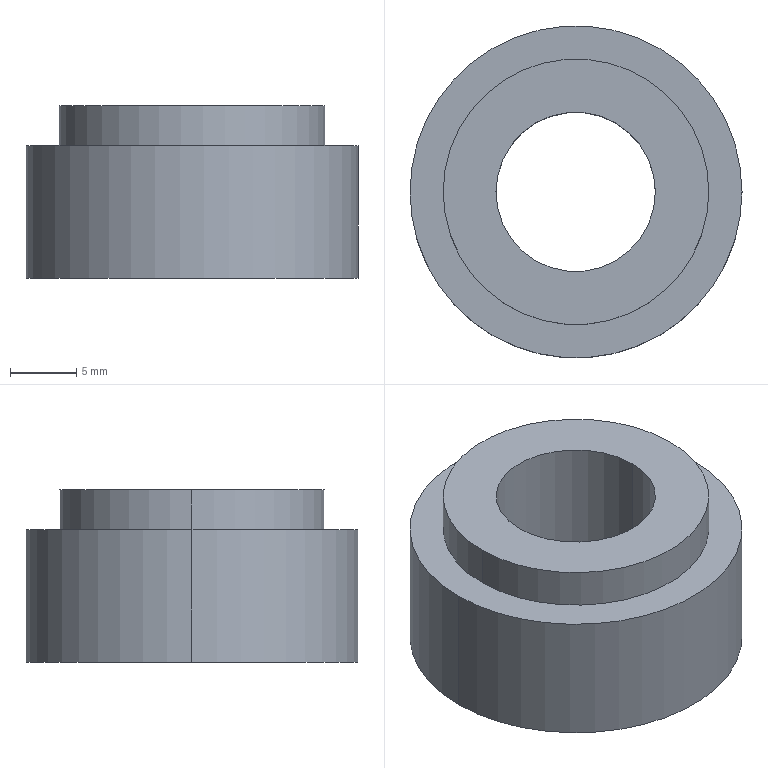Part | SolidWorks | features 3DProfileFeature 1, Extrusion 1, HoleWzd 1, ICE 1 | 1 solid | 9 faces | box 25 x 25 x 13 mm | volume 4381 mm3 | cylinder 6 | plane 3 | commonest cylinder face diameters 12 x2 20 x2 25 x2
STEP:
#1=CARTESIAN_POINT('',(-6.025,-0.002987,0.));
#2=VERTEX_POINT('',#1);
#3=CARTESIAN_POINT('',(5.975,-0.002987,0.));
#4=VERTEX_POINT('',#3);
#5=CARTESIAN_POINT('',(-0.02494,-0.002987,0.));
#6=DIRECTION('',(0.,0.,1.));
#7=DIRECTION('',(1.,0.,0.));
#8=AXIS2_PLACEMENT_3D('',#5,#6,#7);
#9=CIRCLE('',#8,6.);
#10=EDGE_CURVE('',#2,#4,#9,.T.);
#11=ORIENTED_EDGE('',*,*,#10,.F.);
#12=CARTESIAN_POINT('',(-6.025,-0.002987,13.));
#13=VERTEX_POINT('',#12);
#14=CARTESIAN_POINT('',(-6.025,-0.002987,13.));
#15=DIRECTION('',(0.,0.,1.));
#16=VECTOR('',#15,1000.);
#17=LINE('',#14,#16);
#18=EDGE_CURVE('',#2,#13,#17,.T.);
#19=ORIENTED_EDGE('',*,*,#18,.T.);
#20=CARTESIAN_POINT('',(5.975,-0.002987,13.));
#21=VERTEX_POINT('',#20);
#22=CARTESIAN_POINT('',(-0.02494,-0.002987,13.));
#23=DIRECTION('',(0.,0.,1.));
#24=DIRECTION('',(1.,0.,0.));
#25=AXIS2_PLACEMENT_3D('',#22,#23,#24);
#26=CIRCLE('',#25,6.);
#27=EDGE_CURVE('',#13,#21,#26,.T.);
#28=ORIENTED_EDGE('',*,*,#27,.T.);
#29=CARTESIAN_POINT('',(5.975,-0.002987,13.));
#30=DIRECTION('',(0.,0.,1.));
#31=VECTOR('',#30,1000.);
#32=LINE('',#29,#31);
#33=EDGE_CURVE('',#4,#21,#32,.T.);
#34=ORIENTED_EDGE('',*,*,#33,.F.);
#35=EDGE_LOOP('',(#11,#19,#28,#34));
#36=FACE_OUTER_BOUND('',#35,.T.);
#37=CARTESIAN_POINT('',(-0.02494,-0.002987,13.));
#38=DIRECTION('',(0.,0.,1.));
#39=DIRECTION('',(1.,0.,0.));
#40=AXIS2_PLACEMENT_3D('',#37,#38,#39);
#41=CYLINDRICAL_SURFACE('',#40,6.);
#42=ADVANCED_FACE('',(#36),#41,.F.);
#43=CARTESIAN_POINT('',(10.,0.,13.));
#44=VERTEX_POINT('',#43);
#45=CARTESIAN_POINT('',(-10.,0.,13.));
#46=VERTEX_POINT('',#45);
#47=CARTESIAN_POINT('',(0.,0.,13.));
#48=DIRECTION('',(0.,0.,1.));
#49=DIRECTION('',(1.,0.,0.));
#50=AXIS2_PLACEMENT_3D('',#47,#48,#49);
#51=CIRCLE('',#50,10.);
#52=EDGE_CURVE('',#44,#46,#51,.T.);
#53=ORIENTED_EDGE('',*,*,#52,.F.);
#54=CARTESIAN_POINT('',(10.,0.,10.));
#55=VERTEX_POINT('',#54);
#56=CARTESIAN_POINT('',(10.,0.,13.));
#57=DIRECTION('',(0.,0.,-1.));
#58=VECTOR('',#57,1000.);
#59=LINE('',#56,#58);
#60=EDGE_CURVE('',#44,#55,#59,.T.);
#61=ORIENTED_EDGE('',*,*,#60,.T.);
#62=CARTESIAN_POINT('',(-10.,0.,10.));
#63=VERTEX_POINT('',#62);
#64=CARTESIAN_POINT('',(0.,0.,10.));
#65=DIRECTION('',(0.,0.,1.));
#66=DIRECTION('',(1.,0.,0.));
#67=AXIS2_PLACEMENT_3D('',#64,#65,#66);
#68=CIRCLE('',#67,10.);
#69=EDGE_CURVE('',#55,#63,#68,.T.);
#70=ORIENTED_EDGE('',*,*,#69,.T.);
#71=CARTESIAN_POINT('',(-10.,0.,13.));
#72=DIRECTION('',(0.,0.,-1.));
#73=VECTOR('',#72,1000.);
#74=LINE('',#71,#73);
#75=EDGE_CURVE('',#46,#63,#74,.T.);
#76=ORIENTED_EDGE('',*,*,#75,.F.);
#77=EDGE_LOOP('',(#53,#61,#70,#76));
#78=FACE_OUTER_BOUND('',#77,.T.);
#79=CARTESIAN_POINT('',(0.,0.,13.));
#80=DIRECTION('',(0.,0.,-1.));
#81=DIRECTION('',(-1.,0.,0.));
#82=AXIS2_PLACEMENT_3D('',#79,#80,#81);
#83=CYLINDRICAL_SURFACE('',#82,10.);
#84=ADVANCED_FACE('',(#78),#83,.T.);
#85=CARTESIAN_POINT('',(12.5,0.,10.));
#86=VERTEX_POINT('',#85);
#87=CARTESIAN_POINT('',(-12.5,0.,10.));
#88=VERTEX_POINT('',#87);
#89=CARTESIAN_POINT('',(0.,0.,10.));
#90=DIRECTION('',(0.,0.,1.));
#91=DIRECTION('',(1.,0.,0.));
#92=AXIS2_PLACEMENT_3D('',#89,#90,#91);
#93=CIRCLE('',#92,12.5);
#94=EDGE_CURVE('',#86,#88,#93,.T.);
#95=ORIENTED_EDGE('',*,*,#94,.F.);
#96=CARTESIAN_POINT('',(12.5,0.,0.));
#97=VERTEX_POINT('',#96);
#98=CARTESIAN_POINT('',(12.5,0.,10.));
#99=DIRECTION('',(0.,0.,-1.));
#100=VECTOR('',#99,1000.);
#101=LINE('',#98,#100);
#102=EDGE_CURVE('',#86,#97,#101,.T.);
#103=ORIENTED_EDGE('',*,*,#102,.T.);
#104=CARTESIAN_POINT('',(-12.5,0.,0.));
#105=VERTEX_POINT('',#104);
#106=CARTESIAN_POINT('',(0.,0.,0.));
#107=DIRECTION('',(0.,0.,1.));
#108=DIRECTION('',(1.,0.,0.));
#109=AXIS2_PLACEMENT_3D('',#106,#107,#108);
#110=CIRCLE('',#109,12.5);
#111=EDGE_CURVE('',#97,#105,#110,.T.);
#112=ORIENTED_EDGE('',*,*,#111,.T.);
#113=CARTESIAN_POINT('',(-12.5,0.,10.));
#114=DIRECTION('',(0.,0.,-1.));
#115=VECTOR('',#114,1000.);
#116=LINE('',#113,#115);
#117=EDGE_CURVE('',#88,#105,#116,.T.);
#118=ORIENTED_EDGE('',*,*,#117,.F.);
#119=EDGE_LOOP('',(#95,#103,#112,#118));
#120=FACE_OUTER_BOUND('',#119,.T.);
#121=CARTESIAN_POINT('',(0.,0.,10.));
#122=DIRECTION('',(0.,0.,-1.));
#123=DIRECTION('',(-1.,0.,0.));
#124=AXIS2_PLACEMENT_3D('',#121,#122,#123);
#125=CYLINDRICAL_SURFACE('',#124,12.5);
#126=ADVANCED_FACE('',(#120),#125,.T.);
#127=CARTESIAN_POINT('',(0.,0.,10.));
#128=DIRECTION('',(0.,0.,1.));
#129=DIRECTION('',(1.,0.,0.));
#130=AXIS2_PLACEMENT_3D('',#127,#128,#129);
#131=CIRCLE('',#130,12.5);
#132=EDGE_CURVE('',#88,#86,#131,.T.);
#133=ORIENTED_EDGE('',*,*,#132,.T.);
#134=ORIENTED_EDGE('',*,*,#94,.T.);
#135=EDGE_LOOP('',(#133,#134));
#136=FACE_OUTER_BOUND('',#135,.T.);
#137=CARTESIAN_POINT('',(0.,0.,10.));
#138=DIRECTION('',(0.,0.,1.));
#139=DIRECTION('',(1.,0.,0.));
#140=AXIS2_PLACEMENT_3D('',#137,#138,#139);
#141=CIRCLE('',#140,10.);
#142=EDGE_CURVE('',#63,#55,#141,.T.);
#143=ORIENTED_EDGE('',*,*,#142,.F.);
#144=ORIENTED_EDGE('',*,*,#69,.F.);
#145=EDGE_LOOP('',(#143,#144));
#146=FACE_BOUND('',#145,.T.);
#147=CARTESIAN_POINT('',(0.,0.,10.));
#148=DIRECTION('',(0.,0.,1.));
#149=DIRECTION('',(1.,0.,0.));
#150=AXIS2_PLACEMENT_3D('',#147,#148,#149);
#151=PLANE('',#150);
#152=ADVANCED_FACE('',(#136,#146),#151,.T.);
#153=ORIENTED_EDGE('',*,*,#102,.F.);
#154=ORIENTED_EDGE('',*,*,#132,.F.);
#155=ORIENTED_EDGE('',*,*,#117,.T.);
#156=CARTESIAN_POINT('',(0.,0.,0.));
#157=DIRECTION('',(0.,0.,1.));
#158=DIRECTION('',(1.,0.,0.));
#159=AXIS2_PLACEMENT_3D('',#156,#157,#158);
#160=CIRCLE('',#159,12.5);
#161=EDGE_CURVE('',#105,#97,#160,.T.);
#162=ORIENTED_EDGE('',*,*,#161,.T.);
#163=EDGE_LOOP('',(#153,#154,#155,#162));
#164=FACE_OUTER_BOUND('',#163,.T.);
#165=CARTESIAN_POINT('',(0.,0.,10.));
#166=DIRECTION('',(0.,0.,-1.));
#167=DIRECTION('',(-1.,0.,0.));
#168=AXIS2_PLACEMENT_3D('',#165,#166,#167);
#169=CYLINDRICAL_SURFACE('',#168,12.5);
#170=ADVANCED_FACE('',(#164),#169,.T.);
#171=CARTESIAN_POINT('',(-0.02494,-0.002987,0.));
#172=DIRECTION('',(0.,0.,1.));
#173=DIRECTION('',(1.,0.,0.));
#174=AXIS2_PLACEMENT_3D('',#171,#172,#173);
#175=CIRCLE('',#174,6.);
#176=EDGE_CURVE('',#4,#2,#175,.T.);
#177=ORIENTED_EDGE('',*,*,#176,.T.);
#178=ORIENTED_EDGE('',*,*,#10,.T.);
#179=EDGE_LOOP('',(#177,#178));
#180=FACE_BOUND('',#179,.T.);
#181=ORIENTED_EDGE('',*,*,#161,.F.);
#182=ORIENTED_EDGE('',*,*,#111,.F.);
#183=EDGE_LOOP('',(#181,#182));
#184=FACE_OUTER_BOUND('',#183,.T.);
#185=CARTESIAN_POINT('',(0.,0.,0.));
#186=DIRECTION('',(0.,0.,1.));
#187=DIRECTION('',(1.,0.,0.));
#188=AXIS2_PLACEMENT_3D('',#185,#186,#187);
#189=PLANE('',#188);
#190=ADVANCED_FACE('',(#180,#184),#189,.F.);
#191=ORIENTED_EDGE('',*,*,#60,.F.);
#192=CARTESIAN_POINT('',(0.,0.,13.));
#193=DIRECTION('',(0.,0.,1.));
#194=DIRECTION('',(1.,0.,0.));
#195=AXIS2_PLACEMENT_3D('',#192,#193,#194);
#196=CIRCLE('',#195,10.);
#197=EDGE_CURVE('',#46,#44,#196,.T.);
#198=ORIENTED_EDGE('',*,*,#197,.F.);
#199=ORIENTED_EDGE('',*,*,#75,.T.);
#200=ORIENTED_EDGE('',*,*,#142,.T.);
#201=EDGE_LOOP('',(#191,#198,#199,#200));
#202=FACE_OUTER_BOUND('',#201,.T.);
#203=CARTESIAN_POINT('',(0.,0.,13.));
#204=DIRECTION('',(0.,0.,-1.));
#205=DIRECTION('',(-1.,0.,0.));
#206=AXIS2_PLACEMENT_3D('',#203,#204,#205);
#207=CYLINDRICAL_SURFACE('',#206,10.);
#208=ADVANCED_FACE('',(#202),#207,.T.);
#209=CARTESIAN_POINT('',(-0.02494,-0.002987,13.));
#210=DIRECTION('',(0.,0.,1.));
#211=DIRECTION('',(1.,0.,0.));
#212=AXIS2_PLACEMENT_3D('',#209,#210,#211);
#213=CIRCLE('',#212,6.);
#214=EDGE_CURVE('',#21,#13,#213,.T.);
#215=ORIENTED_EDGE('',*,*,#214,.F.);
#216=ORIENTED_EDGE('',*,*,#27,.F.);
#217=EDGE_LOOP('',(#215,#216));
#218=FACE_BOUND('',#217,.T.);
#219=ORIENTED_EDGE('',*,*,#197,.T.);
#220=ORIENTED_EDGE('',*,*,#52,.T.);
#221=EDGE_LOOP('',(#219,#220));
#222=FACE_OUTER_BOUND('',#221,.T.);
#223=CARTESIAN_POINT('',(0.,0.,13.));
#224=DIRECTION('',(0.,0.,1.));
#225=DIRECTION('',(1.,0.,0.));
#226=AXIS2_PLACEMENT_3D('',#223,#224,#225);
#227=PLANE('',#226);
#228=ADVANCED_FACE('',(#218,#222),#227,.T.);
#229=ORIENTED_EDGE('',*,*,#18,.F.);
#230=ORIENTED_EDGE('',*,*,#176,.F.);
#231=ORIENTED_EDGE('',*,*,#33,.T.);
#232=ORIENTED_EDGE('',*,*,#214,.T.);
#233=EDGE_LOOP('',(#229,#230,#231,#232));
#234=FACE_OUTER_BOUND('',#233,.T.);
#235=CARTESIAN_POINT('',(-0.02494,-0.002987,13.));
#236=DIRECTION('',(0.,0.,1.));
#237=DIRECTION('',(1.,0.,0.));
#238=AXIS2_PLACEMENT_3D('',#235,#236,#237);
#239=CYLINDRICAL_SURFACE('',#238,6.);
#240=ADVANCED_FACE('',(#234),#239,.F.);
#241=CLOSED_SHELL('',(#42,#84,#126,#152,#170,#190,#208,#228,#240));
#242=MANIFOLD_SOLID_BREP('',#241);
#243=CARTESIAN_POINT('',(0.,0.,0.));
#244=DIRECTION('',(0.,0.,1.));
#245=DIRECTION('',(1.,0.,0.));
#246=AXIS2_PLACEMENT_3D('',#243,#244,#245);
#247=(LENGTH_UNIT()NAMED_UNIT(*)SI_UNIT(.MILLI.,.METRE.));
#248=UNCERTAINTY_MEASURE_WITH_UNIT(LENGTH_MEASURE(0.00001),#247,'','');
#249=(NAMED_UNIT(*)PLANE_ANGLE_UNIT()SI_UNIT($,.RADIAN.));
#250=(NAMED_UNIT(*)SI_UNIT($,.STERADIAN.)SOLID_ANGLE_UNIT());
#251=(GEOMETRIC_REPRESENTATION_CONTEXT(3)GLOBAL_UNCERTAINTY_ASSIGNED_CONTEXT((#248))GLOBAL_UNIT_ASSIGNED_CONTEXT((#247,#249,#250))REPRESENTATION_CONTEXT('',''));
#252=ADVANCED_BREP_SHAPE_REPRESENTATION('',(#242,#246),#251);